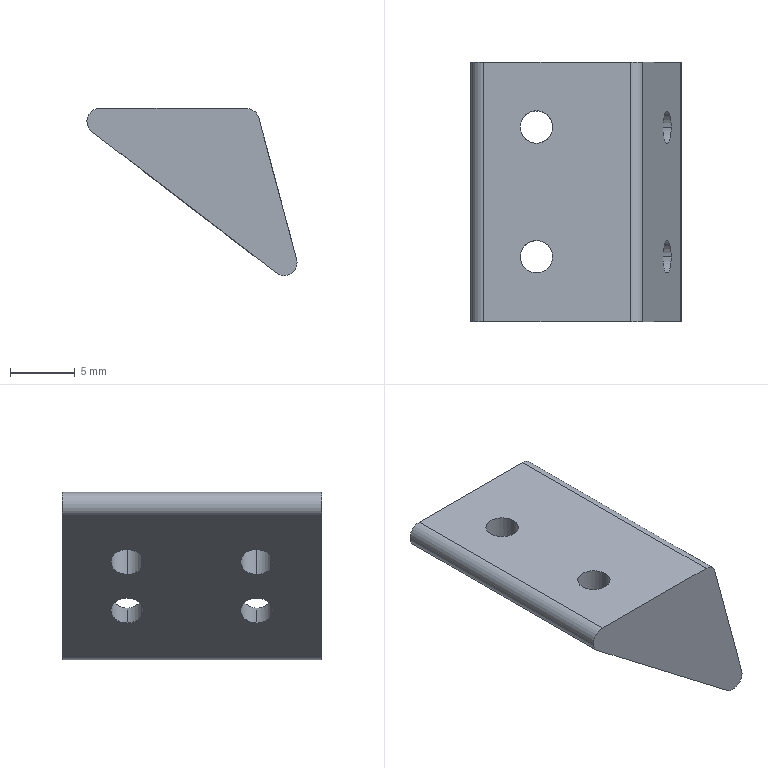Part | SolidWorks | features Extrusion 1, Fillet 1, HoleWzd 1, MirrorPattern 1 | 1 solid | 17 faces | box 16.208 x 20 x 12.902 mm | volume 1998 mm3 | cylinder 12 | plane 5 | commonest cylinder face diameters 2.5 x8 2 x4
STEP:
#1=CARTESIAN_POINT('',(17.154,20.,-12.902));
#2=VERTEX_POINT('',#1);
#3=CARTESIAN_POINT('',(16.545,20.,-12.696));
#4=VERTEX_POINT('',#3);
#5=CARTESIAN_POINT('',(17.154,20.,-11.902));
#6=DIRECTION('',(0.,1.,0.));
#7=DIRECTION('',(0.,0.,1.));
#8=AXIS2_PLACEMENT_3D('',#5,#6,#7);
#9=CIRCLE('',#8,1.);
#10=EDGE_CURVE('',#2,#4,#9,.T.);
#11=ORIENTED_EDGE('',*,*,#10,.F.);
#12=CARTESIAN_POINT('',(17.154,0.,-12.902));
#13=VERTEX_POINT('',#12);
#14=CARTESIAN_POINT('',(17.154,20.,-12.902));
#15=DIRECTION('',(0.,-1.,0.));
#16=VECTOR('',#15,1000.);
#17=LINE('',#14,#16);
#18=EDGE_CURVE('',#2,#13,#17,.T.);
#19=ORIENTED_EDGE('',*,*,#18,.T.);
#20=CARTESIAN_POINT('',(16.545,0.,-12.696));
#21=VERTEX_POINT('',#20);
#22=CARTESIAN_POINT('',(17.154,0.,-11.902));
#23=DIRECTION('',(0.,-1.,0.));
#24=DIRECTION('',(0.,0.,1.));
#25=AXIS2_PLACEMENT_3D('',#22,#23,#24);
#26=CIRCLE('',#25,1.);
#27=EDGE_CURVE('',#21,#13,#26,.T.);
#28=ORIENTED_EDGE('',*,*,#27,.F.);
#29=CARTESIAN_POINT('',(16.545,20.,-12.696));
#30=DIRECTION('',(0.,-1.,0.));
#31=VECTOR('',#30,1000.);
#32=LINE('',#29,#31);
#33=EDGE_CURVE('',#4,#21,#32,.T.);
#34=ORIENTED_EDGE('',*,*,#33,.F.);
#35=EDGE_LOOP('',(#11,#19,#28,#34));
#36=FACE_OUTER_BOUND('',#35,.T.);
#37=CARTESIAN_POINT('',(17.154,20.,-11.902));
#38=DIRECTION('',(0.,-1.,0.));
#39=DIRECTION('',(0.,0.,-1.));
#40=AXIS2_PLACEMENT_3D('',#37,#38,#39);
#41=CYLINDRICAL_SURFACE('',#40,1.);
#42=ADVANCED_FACE('',(#36),#41,.T.);
#43=CARTESIAN_POINT('',(5.75,15.,-4.412));
#44=VERTEX_POINT('',#43);
#45=CARTESIAN_POINT('',(8.25,15.,-6.33));
#46=VERTEX_POINT('',#45);
#47=CARTESIAN_POINT('',(5.75,15.,-4.412));
#48=CARTESIAN_POINT('',(5.75,12.5,-4.412));
#49=CARTESIAN_POINT('',(8.25,12.5,-6.33));
#50=CARTESIAN_POINT('',(8.25,15.,-6.33));
#51=(BOUNDED_CURVE()B_SPLINE_CURVE(3,(#47,#48,#49,#50),.UNSPECIFIED.,.F.,.F.)B_SPLINE_CURVE_WITH_KNOTS((4,4),(0.,3.142),.UNSPECIFIED.)CURVE()GEOMETRIC_REPRESENTATION_ITEM()RATIONAL_B_SPLINE_CURVE((1.,0.3333,0.3333,1.))REPRESENTATION_ITEM(''));
#52=EDGE_CURVE('',#44,#46,#51,.T.);
#53=ORIENTED_EDGE('',*,*,#52,.F.);
#54=CARTESIAN_POINT('',(5.75,15.,0.));
#55=VERTEX_POINT('',#54);
#56=CARTESIAN_POINT('',(5.75,15.,0.));
#57=DIRECTION('',(0.,0.,1.));
#58=VECTOR('',#57,1000.);
#59=LINE('',#56,#58);
#60=EDGE_CURVE('',#44,#55,#59,.T.);
#61=ORIENTED_EDGE('',*,*,#60,.T.);
#62=CARTESIAN_POINT('',(8.25,15.,0.));
#63=VERTEX_POINT('',#62);
#64=CARTESIAN_POINT('',(7.,15.,0.));
#65=DIRECTION('',(0.,0.,1.));
#66=DIRECTION('',(1.,0.,0.));
#67=AXIS2_PLACEMENT_3D('',#64,#65,#66);
#68=CIRCLE('',#67,1.25);
#69=EDGE_CURVE('',#55,#63,#68,.T.);
#70=ORIENTED_EDGE('',*,*,#69,.T.);
#71=CARTESIAN_POINT('',(8.25,15.,0.));
#72=DIRECTION('',(0.,0.,1.));
#73=VECTOR('',#72,1000.);
#74=LINE('',#71,#73);
#75=EDGE_CURVE('',#46,#63,#74,.T.);
#76=ORIENTED_EDGE('',*,*,#75,.F.);
#77=EDGE_LOOP('',(#53,#61,#70,#76));
#78=FACE_OUTER_BOUND('',#77,.T.);
#79=CARTESIAN_POINT('',(7.,15.,0.));
#80=DIRECTION('',(0.,0.,1.));
#81=DIRECTION('',(1.,0.,0.));
#82=AXIS2_PLACEMENT_3D('',#79,#80,#81);
#83=CYLINDRICAL_SURFACE('',#82,1.25);
#84=ADVANCED_FACE('',(#78),#83,.F.);
#85=CARTESIAN_POINT('',(5.75,5.,-4.412));
#86=VERTEX_POINT('',#85);
#87=CARTESIAN_POINT('',(8.25,5.,-6.33));
#88=VERTEX_POINT('',#87);
#89=CARTESIAN_POINT('',(5.75,5.,-4.412));
#90=CARTESIAN_POINT('',(5.75,2.5,-4.412));
#91=CARTESIAN_POINT('',(8.25,2.5,-6.33));
#92=CARTESIAN_POINT('',(8.25,5.,-6.33));
#93=(BOUNDED_CURVE()B_SPLINE_CURVE(3,(#89,#90,#91,#92),.UNSPECIFIED.,.F.,.F.)B_SPLINE_CURVE_WITH_KNOTS((4,4),(0.,3.142),.UNSPECIFIED.)CURVE()GEOMETRIC_REPRESENTATION_ITEM()RATIONAL_B_SPLINE_CURVE((1.,0.3333,0.3333,1.))REPRESENTATION_ITEM(''));
#94=EDGE_CURVE('',#86,#88,#93,.T.);
#95=ORIENTED_EDGE('',*,*,#94,.F.);
#96=CARTESIAN_POINT('',(5.75,5.,0.));
#97=VERTEX_POINT('',#96);
#98=CARTESIAN_POINT('',(5.75,5.,0.));
#99=DIRECTION('',(0.,0.,1.));
#100=VECTOR('',#99,1000.);
#101=LINE('',#98,#100);
#102=EDGE_CURVE('',#86,#97,#101,.T.);
#103=ORIENTED_EDGE('',*,*,#102,.T.);
#104=CARTESIAN_POINT('',(8.25,5.,0.));
#105=VERTEX_POINT('',#104);
#106=CARTESIAN_POINT('',(7.,5.,0.));
#107=DIRECTION('',(0.,0.,1.));
#108=DIRECTION('',(1.,0.,0.));
#109=AXIS2_PLACEMENT_3D('',#106,#107,#108);
#110=CIRCLE('',#109,1.25);
#111=EDGE_CURVE('',#97,#105,#110,.T.);
#112=ORIENTED_EDGE('',*,*,#111,.T.);
#113=CARTESIAN_POINT('',(8.25,5.,0.));
#114=DIRECTION('',(0.,0.,1.));
#115=VECTOR('',#114,1000.);
#116=LINE('',#113,#115);
#117=EDGE_CURVE('',#88,#105,#116,.T.);
#118=ORIENTED_EDGE('',*,*,#117,.F.);
#119=EDGE_LOOP('',(#95,#103,#112,#118));
#120=FACE_OUTER_BOUND('',#119,.T.);
#121=CARTESIAN_POINT('',(7.,5.,0.));
#122=DIRECTION('',(0.,0.,1.));
#123=DIRECTION('',(1.,0.,0.));
#124=AXIS2_PLACEMENT_3D('',#121,#122,#123);
#125=CYLINDRICAL_SURFACE('',#124,1.25);
#126=ADVANCED_FACE('',(#120),#125,.F.);
#127=CARTESIAN_POINT('',(10.632,15.,-8.158));
#128=VERTEX_POINT('',#127);
#129=CARTESIAN_POINT('',(13.132,15.,-10.077));
#130=VERTEX_POINT('',#129);
#131=CARTESIAN_POINT('',(10.632,15.,-8.158));
#132=CARTESIAN_POINT('',(10.632,12.5,-8.158));
#133=CARTESIAN_POINT('',(13.132,12.5,-10.077));
#134=CARTESIAN_POINT('',(13.132,15.,-10.077));
#135=(BOUNDED_CURVE()B_SPLINE_CURVE(3,(#131,#132,#133,#134),.UNSPECIFIED.,.F.,.F.)B_SPLINE_CURVE_WITH_KNOTS((4,4),(3.142,6.283),.UNSPECIFIED.)CURVE()GEOMETRIC_REPRESENTATION_ITEM()RATIONAL_B_SPLINE_CURVE((1.,0.3333,0.3333,1.))REPRESENTATION_ITEM(''));
#136=EDGE_CURVE('',#128,#130,#135,.T.);
#137=ORIENTED_EDGE('',*,*,#136,.F.);
#138=CARTESIAN_POINT('',(16.747,15.,-6.52));
#139=VERTEX_POINT('',#138);
#140=CARTESIAN_POINT('',(16.747,15.,-6.52));
#141=DIRECTION('',(0.9659,0.,0.2588));
#142=VECTOR('',#141,1000.);
#143=LINE('',#140,#142);
#144=EDGE_CURVE('',#128,#139,#143,.T.);
#145=ORIENTED_EDGE('',*,*,#144,.T.);
#146=CARTESIAN_POINT('',(17.394,15.,-8.935));
#147=VERTEX_POINT('',#146);
#148=CARTESIAN_POINT('',(17.071,15.,-7.727));
#149=DIRECTION('',(0.9659,0.,0.2588));
#150=DIRECTION('',(0.2588,0.,-0.9659));
#151=AXIS2_PLACEMENT_3D('',#148,#149,#150);
#152=CIRCLE('',#151,1.25);
#153=EDGE_CURVE('',#139,#147,#152,.T.);
#154=ORIENTED_EDGE('',*,*,#153,.T.);
#155=CARTESIAN_POINT('',(17.394,15.,-8.935));
#156=DIRECTION('',(0.9659,0.,0.2588));
#157=VECTOR('',#156,1000.);
#158=LINE('',#155,#157);
#159=EDGE_CURVE('',#130,#147,#158,.T.);
#160=ORIENTED_EDGE('',*,*,#159,.F.);
#161=EDGE_LOOP('',(#137,#145,#154,#160));
#162=FACE_OUTER_BOUND('',#161,.T.);
#163=CARTESIAN_POINT('',(17.071,15.,-7.727));
#164=DIRECTION('',(0.9659,0.,0.2588));
#165=DIRECTION('',(0.2588,0.,-0.9659));
#166=AXIS2_PLACEMENT_3D('',#163,#164,#165);
#167=CYLINDRICAL_SURFACE('',#166,1.25);
#168=ADVANCED_FACE('',(#162),#167,.F.);
#169=CARTESIAN_POINT('',(10.632,5.,-8.158));
#170=VERTEX_POINT('',#169);
#171=CARTESIAN_POINT('',(13.132,5.,-10.077));
#172=VERTEX_POINT('',#171);
#173=CARTESIAN_POINT('',(10.632,5.,-8.158));
#174=CARTESIAN_POINT('',(10.632,2.5,-8.158));
#175=CARTESIAN_POINT('',(13.132,2.5,-10.077));
#176=CARTESIAN_POINT('',(13.132,5.,-10.077));
#177=(BOUNDED_CURVE()B_SPLINE_CURVE(3,(#173,#174,#175,#176),.UNSPECIFIED.,.F.,.F.)B_SPLINE_CURVE_WITH_KNOTS((4,4),(3.142,6.283),.UNSPECIFIED.)CURVE()GEOMETRIC_REPRESENTATION_ITEM()RATIONAL_B_SPLINE_CURVE((1.,0.3333,0.3333,1.))REPRESENTATION_ITEM(''));
#178=EDGE_CURVE('',#170,#172,#177,.T.);
#179=ORIENTED_EDGE('',*,*,#178,.F.);
#180=CARTESIAN_POINT('',(16.747,5.,-6.52));
#181=VERTEX_POINT('',#180);
#182=CARTESIAN_POINT('',(16.747,5.,-6.52));
#183=DIRECTION('',(0.9659,0.,0.2588));
#184=VECTOR('',#183,1000.);
#185=LINE('',#182,#184);
#186=EDGE_CURVE('',#170,#181,#185,.T.);
#187=ORIENTED_EDGE('',*,*,#186,.T.);
#188=CARTESIAN_POINT('',(17.394,5.,-8.935));
#189=VERTEX_POINT('',#188);
#190=CARTESIAN_POINT('',(17.071,5.,-7.727));
#191=DIRECTION('',(0.9659,0.,0.2588));
#192=DIRECTION('',(0.2588,0.,-0.9659));
#193=AXIS2_PLACEMENT_3D('',#190,#191,#192);
#194=CIRCLE('',#193,1.25);
#195=EDGE_CURVE('',#181,#189,#194,.T.);
#196=ORIENTED_EDGE('',*,*,#195,.T.);
#197=CARTESIAN_POINT('',(17.394,5.,-8.935));
#198=DIRECTION('',(0.9659,0.,0.2588));
#199=VECTOR('',#198,1000.);
#200=LINE('',#197,#199);
#201=EDGE_CURVE('',#172,#189,#200,.T.);
#202=ORIENTED_EDGE('',*,*,#201,.F.);
#203=EDGE_LOOP('',(#179,#187,#196,#202));
#204=FACE_OUTER_BOUND('',#203,.T.);
#205=CARTESIAN_POINT('',(17.071,5.,-7.727));
#206=DIRECTION('',(0.9659,0.,0.2588));
#207=DIRECTION('',(0.2588,0.,-0.9659));
#208=AXIS2_PLACEMENT_3D('',#205,#206,#207);
#209=CYLINDRICAL_SURFACE('',#208,1.25);
#210=ADVANCED_FACE('',(#204),#209,.F.);
#211=CARTESIAN_POINT('',(8.25,15.,-6.33));
#212=CARTESIAN_POINT('',(8.25,17.5,-6.33));
#213=CARTESIAN_POINT('',(5.75,17.5,-4.412));
#214=CARTESIAN_POINT('',(5.75,15.,-4.412));
#215=(BOUNDED_CURVE()B_SPLINE_CURVE(3,(#211,#212,#213,#214),.UNSPECIFIED.,.F.,.F.)B_SPLINE_CURVE_WITH_KNOTS((4,4),(3.142,6.283),.UNSPECIFIED.)CURVE()GEOMETRIC_REPRESENTATION_ITEM()RATIONAL_B_SPLINE_CURVE((1.,0.3333,0.3333,1.))REPRESENTATION_ITEM(''));
#216=EDGE_CURVE('',#46,#44,#215,.T.);
#217=ORIENTED_EDGE('',*,*,#216,.T.);
#218=ORIENTED_EDGE('',*,*,#52,.T.);
#219=EDGE_LOOP('',(#217,#218));
#220=FACE_BOUND('',#219,.T.);
#221=CARTESIAN_POINT('',(8.25,5.,-6.33));
#222=CARTESIAN_POINT('',(8.25,7.5,-6.33));
#223=CARTESIAN_POINT('',(5.75,7.5,-4.412));
#224=CARTESIAN_POINT('',(5.75,5.,-4.412));
#225=(BOUNDED_CURVE()B_SPLINE_CURVE(3,(#221,#222,#223,#224),.UNSPECIFIED.,.F.,.F.)B_SPLINE_CURVE_WITH_KNOTS((4,4),(3.142,6.283),.UNSPECIFIED.)CURVE()GEOMETRIC_REPRESENTATION_ITEM()RATIONAL_B_SPLINE_CURVE((1.,0.3333,0.3333,1.))REPRESENTATION_ITEM(''));
#226=EDGE_CURVE('',#88,#86,#225,.T.);
#227=ORIENTED_EDGE('',*,*,#226,.T.);
#228=ORIENTED_EDGE('',*,*,#94,.T.);
#229=EDGE_LOOP('',(#227,#228));
#230=FACE_BOUND('',#229,.T.);
#231=CARTESIAN_POINT('',(13.132,15.,-10.077));
#232=CARTESIAN_POINT('',(13.132,17.5,-10.077));
#233=CARTESIAN_POINT('',(10.632,17.5,-8.158));
#234=CARTESIAN_POINT('',(10.632,15.,-8.158));
#235=(BOUNDED_CURVE()B_SPLINE_CURVE(3,(#231,#232,#233,#234),.UNSPECIFIED.,.F.,.T.)B_SPLINE_CURVE_WITH_KNOTS((4,4),(0.,3.142),.UNSPECIFIED.)CURVE()GEOMETRIC_REPRESENTATION_ITEM()RATIONAL_B_SPLINE_CURVE((1.,0.3333,0.3333,1.))REPRESENTATION_ITEM(''));
#236=EDGE_CURVE('',#130,#128,#235,.T.);
#237=ORIENTED_EDGE('',*,*,#236,.T.);
#238=ORIENTED_EDGE('',*,*,#136,.T.);
#239=EDGE_LOOP('',(#237,#238));
#240=FACE_BOUND('',#239,.T.);
#241=CARTESIAN_POINT('',(13.132,5.,-10.077));
#242=CARTESIAN_POINT('',(13.132,7.5,-10.077));
#243=CARTESIAN_POINT('',(10.632,7.5,-8.158));
#244=CARTESIAN_POINT('',(10.632,5.,-8.158));
#245=(BOUNDED_CURVE()B_SPLINE_CURVE(3,(#241,#242,#243,#244),.UNSPECIFIED.,.F.,.F.)B_SPLINE_CURVE_WITH_KNOTS((4,4),(0.,3.142),.UNSPECIFIED.)CURVE()GEOMETRIC_REPRESENTATION_ITEM()RATIONAL_B_SPLINE_CURVE((1.,0.3333,0.3333,1.))REPRESENTATION_ITEM(''));
#246=EDGE_CURVE('',#172,#170,#245,.T.);
#247=ORIENTED_EDGE('',*,*,#246,.T.);
#248=ORIENTED_EDGE('',*,*,#178,.T.);
#249=EDGE_LOOP('',(#247,#248));
#250=FACE_BOUND('',#249,.T.);
#251=CARTESIAN_POINT('',(2.337,0.,-1.793));
#252=VERTEX_POINT('',#251);
#253=CARTESIAN_POINT('',(18.882,0.,-14.489));
#254=DIRECTION('',(-0.7934,0.,0.6088));
#255=VECTOR('',#254,1000.);
#256=LINE('',#253,#255);
#257=EDGE_CURVE('',#21,#252,#256,.T.);
#258=ORIENTED_EDGE('',*,*,#257,.T.);
#259=CARTESIAN_POINT('',(2.337,20.,-1.793));
#260=VERTEX_POINT('',#259);
#261=CARTESIAN_POINT('',(2.337,20.,-1.793));
#262=DIRECTION('',(0.,1.,0.));
#263=VECTOR('',#262,1000.);
#264=LINE('',#261,#263);
#265=EDGE_CURVE('',#252,#260,#264,.T.);
#266=ORIENTED_EDGE('',*,*,#265,.T.);
#267=CARTESIAN_POINT('',(18.882,20.,-14.489));
#268=DIRECTION('',(-0.7934,0.,0.6088));
#269=VECTOR('',#268,1000.);
#270=LINE('',#267,#269);
#271=EDGE_CURVE('',#4,#260,#270,.T.);
#272=ORIENTED_EDGE('',*,*,#271,.F.);
#273=ORIENTED_EDGE('',*,*,#33,.T.);
#274=EDGE_LOOP('',(#258,#266,#272,#273));
#275=FACE_OUTER_BOUND('',#274,.T.);
#276=CARTESIAN_POINT('',(18.882,20.,-14.489));
#277=DIRECTION('',(0.6088,0.,0.7934));
#278=DIRECTION('',(0.7934,0.,-0.6088));
#279=AXIS2_PLACEMENT_3D('',#276,#277,#278);
#280=PLANE('',#279);
#281=ADVANCED_FACE('',(#220,#230,#240,#250,#275),#280,.F.);
#282=CARTESIAN_POINT('',(7.,15.,0.));
#283=DIRECTION('',(0.,0.,1.));
#284=DIRECTION('',(1.,0.,0.));
#285=AXIS2_PLACEMENT_3D('',#282,#283,#284);
#286=CIRCLE('',#285,1.25);
#287=EDGE_CURVE('',#63,#55,#286,.T.);
#288=ORIENTED_EDGE('',*,*,#287,.F.);
#289=ORIENTED_EDGE('',*,*,#69,.F.);
#290=EDGE_LOOP('',(#288,#289));
#291=FACE_BOUND('',#290,.T.);
#292=CARTESIAN_POINT('',(7.,5.,0.));
#293=DIRECTION('',(0.,0.,1.));
#294=DIRECTION('',(1.,0.,0.));
#295=AXIS2_PLACEMENT_3D('',#292,#293,#294);
#296=CIRCLE('',#295,1.25);
#297=EDGE_CURVE('',#105,#97,#296,.T.);
#298=ORIENTED_EDGE('',*,*,#297,.F.);
#299=ORIENTED_EDGE('',*,*,#111,.F.);
#300=EDGE_LOOP('',(#298,#299));
#301=FACE_BOUND('',#300,.T.);
#302=CARTESIAN_POINT('',(2.946,0.,0.));
#303=VERTEX_POINT('',#302);
#304=CARTESIAN_POINT('',(14.233,0.,0.));
#305=VERTEX_POINT('',#304);
#306=CARTESIAN_POINT('',(0.,0.,0.));
#307=DIRECTION('',(1.,0.,0.));
#308=VECTOR('',#307,1000.);
#309=LINE('',#306,#308);
#310=EDGE_CURVE('',#303,#305,#309,.T.);
#311=ORIENTED_EDGE('',*,*,#310,.T.);
#312=CARTESIAN_POINT('',(14.233,20.,0.));
#313=VERTEX_POINT('',#312);
#314=CARTESIAN_POINT('',(14.233,20.,0.));
#315=DIRECTION('',(0.,1.,0.));
#316=VECTOR('',#315,1000.);
#317=LINE('',#314,#316);
#318=EDGE_CURVE('',#305,#313,#317,.T.);
#319=ORIENTED_EDGE('',*,*,#318,.T.);
#320=CARTESIAN_POINT('',(2.946,20.,0.));
#321=VERTEX_POINT('',#320);
#322=CARTESIAN_POINT('',(0.,20.,0.));
#323=DIRECTION('',(1.,0.,0.));
#324=VECTOR('',#323,1000.);
#325=LINE('',#322,#324);
#326=EDGE_CURVE('',#321,#313,#325,.T.);
#327=ORIENTED_EDGE('',*,*,#326,.F.);
#328=CARTESIAN_POINT('',(2.946,20.,0.));
#329=DIRECTION('',(0.,-1.,0.));
#330=VECTOR('',#329,1000.);
#331=LINE('',#328,#330);
#332=EDGE_CURVE('',#321,#303,#331,.T.);
#333=ORIENTED_EDGE('',*,*,#332,.T.);
#334=EDGE_LOOP('',(#311,#319,#327,#333));
#335=FACE_OUTER_BOUND('',#334,.T.);
#336=CARTESIAN_POINT('',(0.,20.,0.));
#337=DIRECTION('',(0.,0.,-1.));
#338=DIRECTION('',(-1.,0.,0.));
#339=AXIS2_PLACEMENT_3D('',#336,#337,#338);
#340=PLANE('',#339);
#341=ADVANCED_FACE('',(#291,#301,#335),#340,.F.);
#342=CARTESIAN_POINT('',(17.071,15.,-7.727));
#343=DIRECTION('',(0.9659,0.,0.2588));
#344=DIRECTION('',(0.2588,0.,-0.9659));
#345=AXIS2_PLACEMENT_3D('',#342,#343,#344);
#346=CIRCLE('',#345,1.25);
#347=EDGE_CURVE('',#147,#139,#346,.T.);
#348=ORIENTED_EDGE('',*,*,#347,.F.);
#349=ORIENTED_EDGE('',*,*,#153,.F.);
#350=EDGE_LOOP('',(#348,#349));
#351=FACE_BOUND('',#350,.T.);
#352=CARTESIAN_POINT('',(17.071,5.,-7.727));
#353=DIRECTION('',(0.9659,0.,0.2588));
#354=DIRECTION('',(0.2588,0.,-0.9659));
#355=AXIS2_PLACEMENT_3D('',#352,#353,#354);
#356=CIRCLE('',#355,1.25);
#357=EDGE_CURVE('',#189,#181,#356,.T.);
#358=ORIENTED_EDGE('',*,*,#357,.F.);
#359=ORIENTED_EDGE('',*,*,#195,.F.);
#360=EDGE_LOOP('',(#358,#359));
#361=FACE_BOUND('',#360,.T.);
#362=CARTESIAN_POINT('',(15.199,20.,-0.7412));
#363=VERTEX_POINT('',#362);
#364=CARTESIAN_POINT('',(18.12,20.,-11.643));
#365=VERTEX_POINT('',#364);
#366=CARTESIAN_POINT('',(15.,20.,0.));
#367=DIRECTION('',(0.2588,0.,-0.9659));
#368=VECTOR('',#367,1000.);
#369=LINE('',#366,#368);
#370=EDGE_CURVE('',#363,#365,#369,.T.);
#371=ORIENTED_EDGE('',*,*,#370,.F.);
#372=CARTESIAN_POINT('',(15.199,0.,-0.7412));
#373=VERTEX_POINT('',#372);
#374=CARTESIAN_POINT('',(15.199,20.,-0.7412));
#375=DIRECTION('',(0.,-1.,0.));
#376=VECTOR('',#375,1000.);
#377=LINE('',#374,#376);
#378=EDGE_CURVE('',#363,#373,#377,.T.);
#379=ORIENTED_EDGE('',*,*,#378,.T.);
#380=CARTESIAN_POINT('',(18.12,0.,-11.643));
#381=VERTEX_POINT('',#380);
#382=CARTESIAN_POINT('',(15.,0.,0.));
#383=DIRECTION('',(0.2588,0.,-0.9659));
#384=VECTOR('',#383,1000.);
#385=LINE('',#382,#384);
#386=EDGE_CURVE('',#373,#381,#385,.T.);
#387=ORIENTED_EDGE('',*,*,#386,.T.);
#388=CARTESIAN_POINT('',(18.12,20.,-11.643));
#389=DIRECTION('',(0.,1.,0.));
#390=VECTOR('',#389,1000.);
#391=LINE('',#388,#390);
#392=EDGE_CURVE('',#381,#365,#391,.T.);
#393=ORIENTED_EDGE('',*,*,#392,.T.);
#394=EDGE_LOOP('',(#371,#379,#387,#393));
#395=FACE_OUTER_BOUND('',#394,.T.);
#396=CARTESIAN_POINT('',(15.,20.,0.));
#397=DIRECTION('',(-0.9659,0.,-0.2588));
#398=DIRECTION('',(-0.2588,0.,0.9659));
#399=AXIS2_PLACEMENT_3D('',#396,#397,#398);
#400=PLANE('',#399);
#401=ADVANCED_FACE('',(#351,#361,#395),#400,.F.);
#402=ORIENTED_EDGE('',*,*,#326,.T.);
#403=CARTESIAN_POINT('',(14.233,20.,-1.));
#404=DIRECTION('',(0.,1.,0.));
#405=DIRECTION('',(0.,0.,1.));
#406=AXIS2_PLACEMENT_3D('',#403,#404,#405);
#407=CIRCLE('',#406,1.);
#408=EDGE_CURVE('',#313,#363,#407,.T.);
#409=ORIENTED_EDGE('',*,*,#408,.T.);
#410=ORIENTED_EDGE('',*,*,#370,.T.);
#411=CARTESIAN_POINT('',(17.154,20.,-11.902));
#412=DIRECTION('',(0.,1.,0.));
#413=DIRECTION('',(0.,0.,1.));
#414=AXIS2_PLACEMENT_3D('',#411,#412,#413);
#415=CIRCLE('',#414,1.);
#416=EDGE_CURVE('',#365,#2,#415,.T.);
#417=ORIENTED_EDGE('',*,*,#416,.T.);
#418=ORIENTED_EDGE('',*,*,#10,.T.);
#419=ORIENTED_EDGE('',*,*,#271,.T.);
#420=CARTESIAN_POINT('',(2.946,20.,-1.));
#421=DIRECTION('',(0.,1.,0.));
#422=DIRECTION('',(0.,0.,1.));
#423=AXIS2_PLACEMENT_3D('',#420,#421,#422);
#424=CIRCLE('',#423,1.);
#425=EDGE_CURVE('',#260,#321,#424,.T.);
#426=ORIENTED_EDGE('',*,*,#425,.T.);
#427=EDGE_LOOP('',(#402,#409,#410,#417,#418,#419,#426));
#428=FACE_OUTER_BOUND('',#427,.T.);
#429=CARTESIAN_POINT('',(0.,20.,0.));
#430=DIRECTION('',(0.,1.,0.));
#431=DIRECTION('',(0.,0.,1.));
#432=AXIS2_PLACEMENT_3D('',#429,#430,#431);
#433=PLANE('',#432);
#434=ADVANCED_FACE('',(#428),#433,.T.);
#435=ORIENTED_EDGE('',*,*,#386,.F.);
#436=CARTESIAN_POINT('',(14.233,0.,-1.));
#437=DIRECTION('',(0.,-1.,0.));
#438=DIRECTION('',(0.,0.,1.));
#439=AXIS2_PLACEMENT_3D('',#436,#437,#438);
#440=CIRCLE('',#439,1.);
#441=EDGE_CURVE('',#373,#305,#440,.T.);
#442=ORIENTED_EDGE('',*,*,#441,.T.);
#443=ORIENTED_EDGE('',*,*,#310,.F.);
#444=CARTESIAN_POINT('',(2.946,0.,-1.));
#445=DIRECTION('',(0.,-1.,0.));
#446=DIRECTION('',(0.,0.,1.));
#447=AXIS2_PLACEMENT_3D('',#444,#445,#446);
#448=CIRCLE('',#447,1.);
#449=EDGE_CURVE('',#303,#252,#448,.T.);
#450=ORIENTED_EDGE('',*,*,#449,.T.);
#451=ORIENTED_EDGE('',*,*,#257,.F.);
#452=ORIENTED_EDGE('',*,*,#27,.T.);
#453=CARTESIAN_POINT('',(17.154,0.,-11.902));
#454=DIRECTION('',(0.,-1.,0.));
#455=DIRECTION('',(0.,0.,1.));
#456=AXIS2_PLACEMENT_3D('',#453,#454,#455);
#457=CIRCLE('',#456,1.);
#458=EDGE_CURVE('',#13,#381,#457,.T.);
#459=ORIENTED_EDGE('',*,*,#458,.T.);
#460=EDGE_LOOP('',(#435,#442,#443,#450,#451,#452,#459));
#461=FACE_OUTER_BOUND('',#460,.T.);
#462=CARTESIAN_POINT('',(0.,0.,0.));
#463=DIRECTION('',(0.,1.,0.));
#464=DIRECTION('',(0.,0.,1.));
#465=AXIS2_PLACEMENT_3D('',#462,#463,#464);
#466=PLANE('',#465);
#467=ADVANCED_FACE('',(#461),#466,.F.);
#468=ORIENTED_EDGE('',*,*,#186,.F.);
#469=ORIENTED_EDGE('',*,*,#246,.F.);
#470=ORIENTED_EDGE('',*,*,#201,.T.);
#471=ORIENTED_EDGE('',*,*,#357,.T.);
#472=EDGE_LOOP('',(#468,#469,#470,#471));
#473=FACE_OUTER_BOUND('',#472,.T.);
#474=CARTESIAN_POINT('',(17.071,5.,-7.727));
#475=DIRECTION('',(0.9659,0.,0.2588));
#476=DIRECTION('',(0.2588,0.,-0.9659));
#477=AXIS2_PLACEMENT_3D('',#474,#475,#476);
#478=CYLINDRICAL_SURFACE('',#477,1.25);
#479=ADVANCED_FACE('',(#473),#478,.F.);
#480=ORIENTED_EDGE('',*,*,#144,.F.);
#481=ORIENTED_EDGE('',*,*,#236,.F.);
#482=ORIENTED_EDGE('',*,*,#159,.T.);
#483=ORIENTED_EDGE('',*,*,#347,.T.);
#484=EDGE_LOOP('',(#480,#481,#482,#483));
#485=FACE_OUTER_BOUND('',#484,.T.);
#486=CARTESIAN_POINT('',(17.071,15.,-7.727));
#487=DIRECTION('',(0.9659,0.,0.2588));
#488=DIRECTION('',(0.2588,0.,-0.9659));
#489=AXIS2_PLACEMENT_3D('',#486,#487,#488);
#490=CYLINDRICAL_SURFACE('',#489,1.25);
#491=ADVANCED_FACE('',(#485),#490,.F.);
#492=ORIENTED_EDGE('',*,*,#102,.F.);
#493=ORIENTED_EDGE('',*,*,#226,.F.);
#494=ORIENTED_EDGE('',*,*,#117,.T.);
#495=ORIENTED_EDGE('',*,*,#297,.T.);
#496=EDGE_LOOP('',(#492,#493,#494,#495));
#497=FACE_OUTER_BOUND('',#496,.T.);
#498=CARTESIAN_POINT('',(7.,5.,0.));
#499=DIRECTION('',(0.,0.,1.));
#500=DIRECTION('',(1.,0.,0.));
#501=AXIS2_PLACEMENT_3D('',#498,#499,#500);
#502=CYLINDRICAL_SURFACE('',#501,1.25);
#503=ADVANCED_FACE('',(#497),#502,.F.);
#504=ORIENTED_EDGE('',*,*,#60,.F.);
#505=ORIENTED_EDGE('',*,*,#216,.F.);
#506=ORIENTED_EDGE('',*,*,#75,.T.);
#507=ORIENTED_EDGE('',*,*,#287,.T.);
#508=EDGE_LOOP('',(#504,#505,#506,#507));
#509=FACE_OUTER_BOUND('',#508,.T.);
#510=CARTESIAN_POINT('',(7.,15.,0.));
#511=DIRECTION('',(0.,0.,1.));
#512=DIRECTION('',(1.,0.,0.));
#513=AXIS2_PLACEMENT_3D('',#510,#511,#512);
#514=CYLINDRICAL_SURFACE('',#513,1.25);
#515=ADVANCED_FACE('',(#509),#514,.F.);
#516=ORIENTED_EDGE('',*,*,#408,.F.);
#517=ORIENTED_EDGE('',*,*,#318,.F.);
#518=ORIENTED_EDGE('',*,*,#441,.F.);
#519=ORIENTED_EDGE('',*,*,#378,.F.);
#520=EDGE_LOOP('',(#516,#517,#518,#519));
#521=FACE_OUTER_BOUND('',#520,.T.);
#522=CARTESIAN_POINT('',(14.233,20.,-1.));
#523=DIRECTION('',(0.,-1.,0.));
#524=DIRECTION('',(0.,0.,-1.));
#525=AXIS2_PLACEMENT_3D('',#522,#523,#524);
#526=CYLINDRICAL_SURFACE('',#525,1.);
#527=ADVANCED_FACE('',(#521),#526,.T.);
#528=ORIENTED_EDGE('',*,*,#425,.F.);
#529=ORIENTED_EDGE('',*,*,#265,.F.);
#530=ORIENTED_EDGE('',*,*,#449,.F.);
#531=ORIENTED_EDGE('',*,*,#332,.F.);
#532=EDGE_LOOP('',(#528,#529,#530,#531));
#533=FACE_OUTER_BOUND('',#532,.T.);
#534=CARTESIAN_POINT('',(2.946,20.,-1.));
#535=DIRECTION('',(0.,-1.,0.));
#536=DIRECTION('',(0.,0.,-1.));
#537=AXIS2_PLACEMENT_3D('',#534,#535,#536);
#538=CYLINDRICAL_SURFACE('',#537,1.);
#539=ADVANCED_FACE('',(#533),#538,.T.);
#540=ORIENTED_EDGE('',*,*,#18,.F.);
#541=ORIENTED_EDGE('',*,*,#416,.F.);
#542=ORIENTED_EDGE('',*,*,#392,.F.);
#543=ORIENTED_EDGE('',*,*,#458,.F.);
#544=EDGE_LOOP('',(#540,#541,#542,#543));
#545=FACE_OUTER_BOUND('',#544,.T.);
#546=CARTESIAN_POINT('',(17.154,20.,-11.902));
#547=DIRECTION('',(0.,-1.,0.));
#548=DIRECTION('',(0.,0.,-1.));
#549=AXIS2_PLACEMENT_3D('',#546,#547,#548);
#550=CYLINDRICAL_SURFACE('',#549,1.);
#551=ADVANCED_FACE('',(#545),#550,.T.);
#552=CLOSED_SHELL('',(#42,#84,#126,#168,#210,#281,#341,#401,#434,#467,#479,#491,#503,#515,#527,#539,#551));
#553=MANIFOLD_SOLID_BREP('',#552);
#554=CARTESIAN_POINT('',(0.,0.,0.));
#555=DIRECTION('',(0.,0.,1.));
#556=DIRECTION('',(1.,0.,0.));
#557=AXIS2_PLACEMENT_3D('',#554,#555,#556);
#558=(LENGTH_UNIT()NAMED_UNIT(*)SI_UNIT(.MILLI.,.METRE.));
#559=UNCERTAINTY_MEASURE_WITH_UNIT(LENGTH_MEASURE(0.00001),#558,'','');
#560=(NAMED_UNIT(*)PLANE_ANGLE_UNIT()SI_UNIT($,.RADIAN.));
#561=(NAMED_UNIT(*)SI_UNIT($,.STERADIAN.)SOLID_ANGLE_UNIT());
#562=(GEOMETRIC_REPRESENTATION_CONTEXT(3)GLOBAL_UNCERTAINTY_ASSIGNED_CONTEXT((#559))GLOBAL_UNIT_ASSIGNED_CONTEXT((#558,#560,#561))REPRESENTATION_CONTEXT('',''));
#563=ADVANCED_BREP_SHAPE_REPRESENTATION('',(#553,#557),#562);